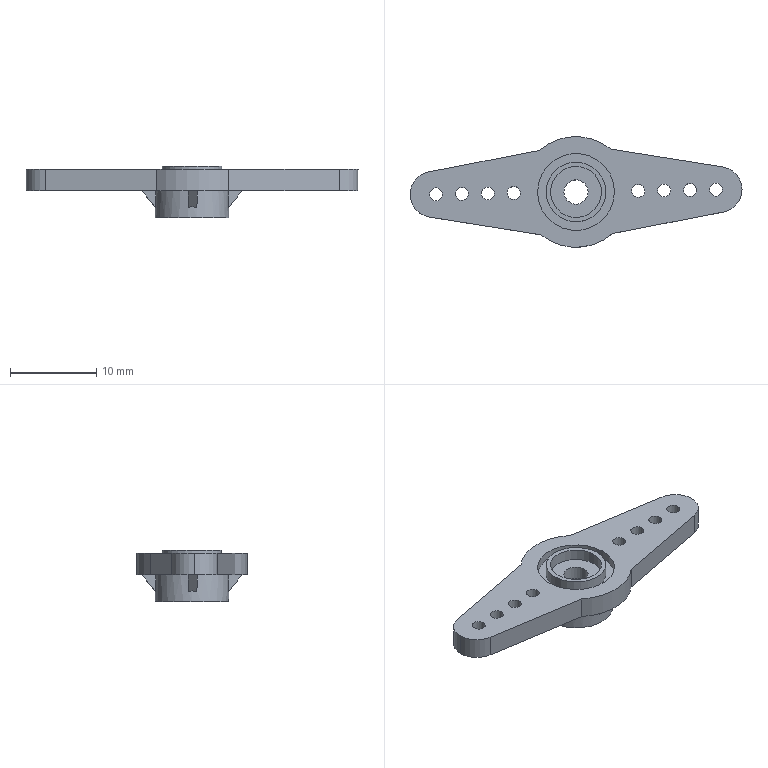Part | STEP file | Zapas-OpenRC Truggy HSPr v2. v55-1_2 | 1 solid | 119 faces | box 38.395 x 12.8 x 5.95 mm | volume 788.17 mm3 | plane 75 | cylinder 44 | commonest cylinder face diameters 5.2 x26 1.5 x8 5.3 x3 12.8 x2 2.8 x1 5.9 x1